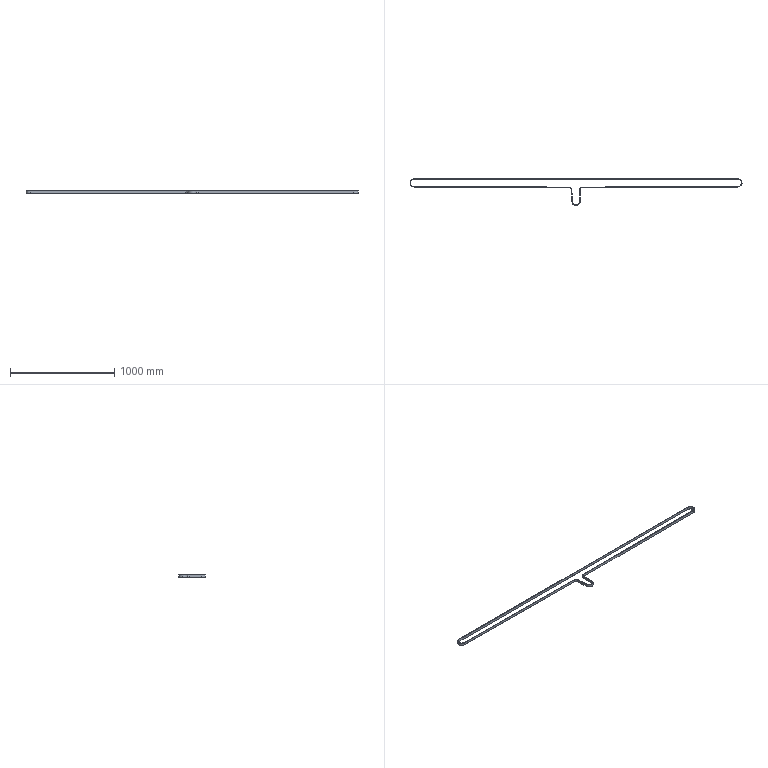Part | STEP file | LTBR-S8M-840^ | 1 solid | 24 faces | box 3180 x 255.872 x 25 mm | volume 890028 mm3 | cylinder 12 | plane 12 | commonest cylinder face diameters 69.36 x4 79.96 x4 39.4 x2 50 x2